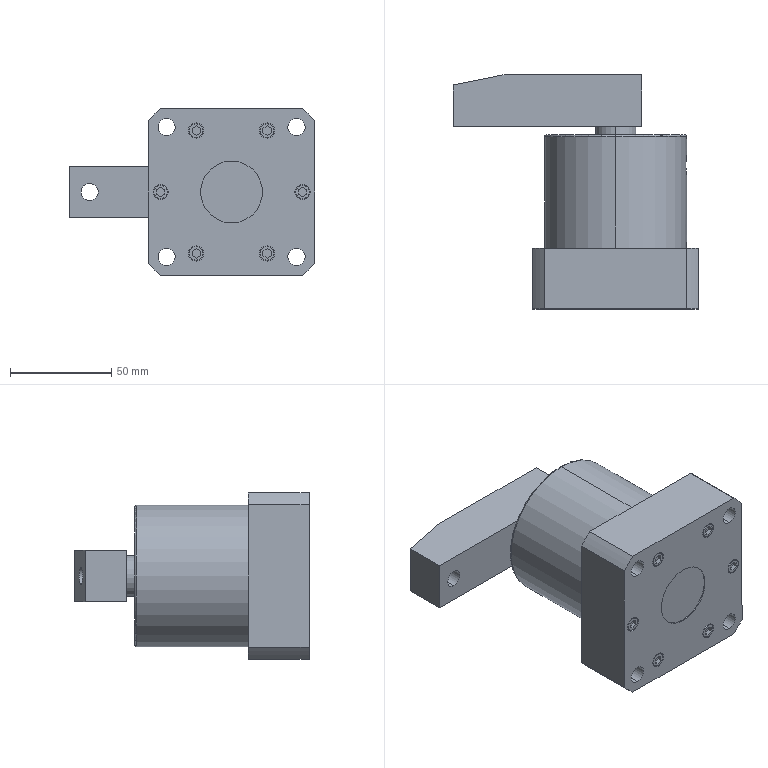Part | SolidWorks | features BaseBody 2, HoleWzd 1, ICE 1 | 2 solids | 159 faces | box 121 x 115.5 x 82 mm | volume 382870 mm3 | plane 75 | cylinder 58 | torus 14 | cone 12 | commonest cylinder face diameters 7 x12 7.5 x12 8.5 x10 8.566 x4 20 x4 108 x4